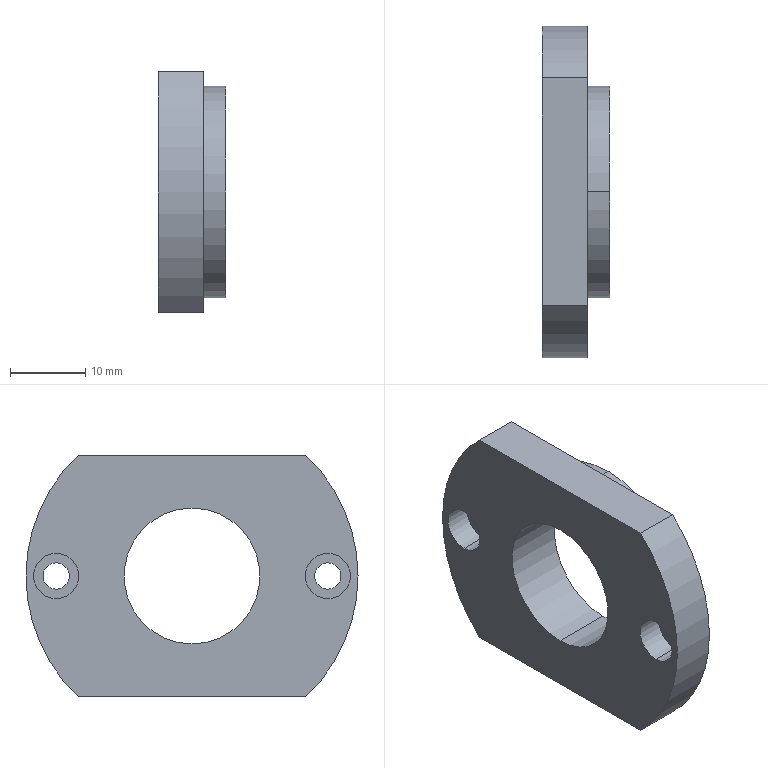Part | SolidWorks | features HoleWzd 1, ICE 1, Revolution 1 | 1 solid | 24 faces | box 9 x 44 x 32 mm | volume 6703 mm3 | cylinder 16 | plane 8 | commonest cylinder face diameters 3.5 x4 6 x4 18 x2 25 x2 28 x2 44 x2
STEP:
#1=CARTESIAN_POINT('',(3.5,18.,-3.));
#2=VERTEX_POINT('',#1);
#3=CARTESIAN_POINT('',(3.5,18.,3.));
#4=VERTEX_POINT('',#3);
#5=CARTESIAN_POINT('',(3.5,18.,0.));
#6=DIRECTION('',(-1.,0.,0.));
#7=DIRECTION('',(0.,0.,1.));
#8=AXIS2_PLACEMENT_3D('',#5,#6,#7);
#9=CIRCLE('',#8,3.);
#10=EDGE_CURVE('',#2,#4,#9,.T.);
#11=ORIENTED_EDGE('',*,*,#10,.F.);
#12=CARTESIAN_POINT('',(0.,18.,-3.));
#13=VERTEX_POINT('',#12);
#14=CARTESIAN_POINT('',(0.,18.,-3.));
#15=DIRECTION('',(-1.,0.,0.));
#16=VECTOR('',#15,1000.);
#17=LINE('',#14,#16);
#18=EDGE_CURVE('',#2,#13,#17,.T.);
#19=ORIENTED_EDGE('',*,*,#18,.T.);
#20=CARTESIAN_POINT('',(0.,18.,3.));
#21=VERTEX_POINT('',#20);
#22=CARTESIAN_POINT('',(0.,18.,0.));
#23=DIRECTION('',(-1.,0.,0.));
#24=DIRECTION('',(0.,0.,1.));
#25=AXIS2_PLACEMENT_3D('',#22,#23,#24);
#26=CIRCLE('',#25,3.);
#27=EDGE_CURVE('',#13,#21,#26,.T.);
#28=ORIENTED_EDGE('',*,*,#27,.T.);
#29=CARTESIAN_POINT('',(0.,18.,3.));
#30=DIRECTION('',(-1.,0.,0.));
#31=VECTOR('',#30,1000.);
#32=LINE('',#29,#31);
#33=EDGE_CURVE('',#4,#21,#32,.T.);
#34=ORIENTED_EDGE('',*,*,#33,.F.);
#35=EDGE_LOOP('',(#11,#19,#28,#34));
#36=FACE_OUTER_BOUND('',#35,.T.);
#37=CARTESIAN_POINT('',(0.,18.,0.));
#38=DIRECTION('',(-1.,0.,0.));
#39=DIRECTION('',(0.,0.,1.));
#40=AXIS2_PLACEMENT_3D('',#37,#38,#39);
#41=CYLINDRICAL_SURFACE('',#40,3.);
#42=ADVANCED_FACE('',(#36),#41,.F.);
#43=CARTESIAN_POINT('',(6.,18.,-1.75));
#44=VERTEX_POINT('',#43);
#45=CARTESIAN_POINT('',(6.,18.,1.75));
#46=VERTEX_POINT('',#45);
#47=CARTESIAN_POINT('',(6.,18.,0.));
#48=DIRECTION('',(-1.,0.,0.));
#49=DIRECTION('',(0.,0.,1.));
#50=AXIS2_PLACEMENT_3D('',#47,#48,#49);
#51=CIRCLE('',#50,1.75);
#52=EDGE_CURVE('',#44,#46,#51,.T.);
#53=ORIENTED_EDGE('',*,*,#52,.F.);
#54=CARTESIAN_POINT('',(3.5,18.,-1.75));
#55=VERTEX_POINT('',#54);
#56=CARTESIAN_POINT('',(0.,18.,-1.75));
#57=DIRECTION('',(-1.,0.,0.));
#58=VECTOR('',#57,1000.);
#59=LINE('',#56,#58);
#60=EDGE_CURVE('',#44,#55,#59,.T.);
#61=ORIENTED_EDGE('',*,*,#60,.T.);
#62=CARTESIAN_POINT('',(3.5,18.,1.75));
#63=VERTEX_POINT('',#62);
#64=CARTESIAN_POINT('',(3.5,18.,0.));
#65=DIRECTION('',(-1.,0.,0.));
#66=DIRECTION('',(0.,0.,1.));
#67=AXIS2_PLACEMENT_3D('',#64,#65,#66);
#68=CIRCLE('',#67,1.75);
#69=EDGE_CURVE('',#55,#63,#68,.T.);
#70=ORIENTED_EDGE('',*,*,#69,.T.);
#71=CARTESIAN_POINT('',(0.,18.,1.75));
#72=DIRECTION('',(-1.,0.,0.));
#73=VECTOR('',#72,1000.);
#74=LINE('',#71,#73);
#75=EDGE_CURVE('',#46,#63,#74,.T.);
#76=ORIENTED_EDGE('',*,*,#75,.F.);
#77=EDGE_LOOP('',(#53,#61,#70,#76));
#78=FACE_OUTER_BOUND('',#77,.T.);
#79=CARTESIAN_POINT('',(0.,18.,0.));
#80=DIRECTION('',(-1.,0.,0.));
#81=DIRECTION('',(0.,0.,1.));
#82=AXIS2_PLACEMENT_3D('',#79,#80,#81);
#83=CYLINDRICAL_SURFACE('',#82,1.75);
#84=ADVANCED_FACE('',(#78),#83,.F.);
#85=CARTESIAN_POINT('',(3.5,-18.,-3.));
#86=VERTEX_POINT('',#85);
#87=CARTESIAN_POINT('',(3.5,-18.,3.));
#88=VERTEX_POINT('',#87);
#89=CARTESIAN_POINT('',(3.5,-18.,0.));
#90=DIRECTION('',(-1.,0.,0.));
#91=DIRECTION('',(0.,0.,1.));
#92=AXIS2_PLACEMENT_3D('',#89,#90,#91);
#93=CIRCLE('',#92,3.);
#94=EDGE_CURVE('',#86,#88,#93,.T.);
#95=ORIENTED_EDGE('',*,*,#94,.F.);
#96=CARTESIAN_POINT('',(0.,-18.,-3.));
#97=VERTEX_POINT('',#96);
#98=CARTESIAN_POINT('',(0.,-18.,-3.));
#99=DIRECTION('',(-1.,0.,0.));
#100=VECTOR('',#99,1000.);
#101=LINE('',#98,#100);
#102=EDGE_CURVE('',#86,#97,#101,.T.);
#103=ORIENTED_EDGE('',*,*,#102,.T.);
#104=CARTESIAN_POINT('',(0.,-18.,3.));
#105=VERTEX_POINT('',#104);
#106=CARTESIAN_POINT('',(0.,-18.,0.));
#107=DIRECTION('',(-1.,0.,0.));
#108=DIRECTION('',(0.,0.,1.));
#109=AXIS2_PLACEMENT_3D('',#106,#107,#108);
#110=CIRCLE('',#109,3.);
#111=EDGE_CURVE('',#97,#105,#110,.T.);
#112=ORIENTED_EDGE('',*,*,#111,.T.);
#113=CARTESIAN_POINT('',(0.,-18.,3.));
#114=DIRECTION('',(-1.,0.,0.));
#115=VECTOR('',#114,1000.);
#116=LINE('',#113,#115);
#117=EDGE_CURVE('',#88,#105,#116,.T.);
#118=ORIENTED_EDGE('',*,*,#117,.F.);
#119=EDGE_LOOP('',(#95,#103,#112,#118));
#120=FACE_OUTER_BOUND('',#119,.T.);
#121=CARTESIAN_POINT('',(0.,-18.,0.));
#122=DIRECTION('',(-1.,0.,0.));
#123=DIRECTION('',(0.,0.,1.));
#124=AXIS2_PLACEMENT_3D('',#121,#122,#123);
#125=CYLINDRICAL_SURFACE('',#124,3.);
#126=ADVANCED_FACE('',(#120),#125,.F.);
#127=CARTESIAN_POINT('',(6.,-18.,-1.75));
#128=VERTEX_POINT('',#127);
#129=CARTESIAN_POINT('',(6.,-18.,1.75));
#130=VERTEX_POINT('',#129);
#131=CARTESIAN_POINT('',(6.,-18.,0.));
#132=DIRECTION('',(-1.,0.,0.));
#133=DIRECTION('',(0.,0.,1.));
#134=AXIS2_PLACEMENT_3D('',#131,#132,#133);
#135=CIRCLE('',#134,1.75);
#136=EDGE_CURVE('',#128,#130,#135,.T.);
#137=ORIENTED_EDGE('',*,*,#136,.F.);
#138=CARTESIAN_POINT('',(3.5,-18.,-1.75));
#139=VERTEX_POINT('',#138);
#140=CARTESIAN_POINT('',(0.,-18.,-1.75));
#141=DIRECTION('',(-1.,0.,0.));
#142=VECTOR('',#141,1000.);
#143=LINE('',#140,#142);
#144=EDGE_CURVE('',#128,#139,#143,.T.);
#145=ORIENTED_EDGE('',*,*,#144,.T.);
#146=CARTESIAN_POINT('',(3.5,-18.,1.75));
#147=VERTEX_POINT('',#146);
#148=CARTESIAN_POINT('',(3.5,-18.,0.));
#149=DIRECTION('',(-1.,0.,0.));
#150=DIRECTION('',(0.,0.,1.));
#151=AXIS2_PLACEMENT_3D('',#148,#149,#150);
#152=CIRCLE('',#151,1.75);
#153=EDGE_CURVE('',#139,#147,#152,.T.);
#154=ORIENTED_EDGE('',*,*,#153,.T.);
#155=CARTESIAN_POINT('',(0.,-18.,1.75));
#156=DIRECTION('',(-1.,0.,0.));
#157=VECTOR('',#156,1000.);
#158=LINE('',#155,#157);
#159=EDGE_CURVE('',#130,#147,#158,.T.);
#160=ORIENTED_EDGE('',*,*,#159,.F.);
#161=EDGE_LOOP('',(#137,#145,#154,#160));
#162=FACE_OUTER_BOUND('',#161,.T.);
#163=CARTESIAN_POINT('',(0.,-18.,0.));
#164=DIRECTION('',(-1.,0.,0.));
#165=DIRECTION('',(0.,0.,1.));
#166=AXIS2_PLACEMENT_3D('',#163,#164,#165);
#167=CYLINDRICAL_SURFACE('',#166,1.75);
#168=ADVANCED_FACE('',(#162),#167,.F.);
#169=CARTESIAN_POINT('',(9.,0.,-12.5));
#170=VERTEX_POINT('',#169);
#171=CARTESIAN_POINT('',(9.,0.,12.5));
#172=VERTEX_POINT('',#171);
#173=CARTESIAN_POINT('',(9.,0.,0.));
#174=DIRECTION('',(-1.,0.,0.));
#175=DIRECTION('',(0.,0.,1.));
#176=AXIS2_PLACEMENT_3D('',#173,#174,#175);
#177=CIRCLE('',#176,12.5);
#178=EDGE_CURVE('',#170,#172,#177,.T.);
#179=ORIENTED_EDGE('',*,*,#178,.F.);
#180=CARTESIAN_POINT('',(8.,0.,-12.5));
#181=VERTEX_POINT('',#180);
#182=CARTESIAN_POINT('',(0.,0.,-12.5));
#183=DIRECTION('',(-1.,0.,0.));
#184=VECTOR('',#183,1000.);
#185=LINE('',#182,#184);
#186=EDGE_CURVE('',#170,#181,#185,.T.);
#187=ORIENTED_EDGE('',*,*,#186,.T.);
#188=CARTESIAN_POINT('',(8.,0.,12.5));
#189=VERTEX_POINT('',#188);
#190=CARTESIAN_POINT('',(8.,0.,0.));
#191=DIRECTION('',(-1.,0.,0.));
#192=DIRECTION('',(0.,0.,1.));
#193=AXIS2_PLACEMENT_3D('',#190,#191,#192);
#194=CIRCLE('',#193,12.5);
#195=EDGE_CURVE('',#181,#189,#194,.T.);
#196=ORIENTED_EDGE('',*,*,#195,.T.);
#197=CARTESIAN_POINT('',(0.,0.,12.5));
#198=DIRECTION('',(-1.,0.,0.));
#199=VECTOR('',#198,1000.);
#200=LINE('',#197,#199);
#201=EDGE_CURVE('',#172,#189,#200,.T.);
#202=ORIENTED_EDGE('',*,*,#201,.F.);
#203=EDGE_LOOP('',(#179,#187,#196,#202));
#204=FACE_OUTER_BOUND('',#203,.T.);
#205=CARTESIAN_POINT('',(0.,0.,0.));
#206=DIRECTION('',(-1.,0.,0.));
#207=DIRECTION('',(0.,0.,1.));
#208=AXIS2_PLACEMENT_3D('',#205,#206,#207);
#209=CYLINDRICAL_SURFACE('',#208,12.5);
#210=ADVANCED_FACE('',(#204),#209,.F.);
#211=CARTESIAN_POINT('',(9.,0.,14.));
#212=VERTEX_POINT('',#211);
#213=CARTESIAN_POINT('',(9.,0.,-14.));
#214=VERTEX_POINT('',#213);
#215=CARTESIAN_POINT('',(9.,0.,0.));
#216=DIRECTION('',(-1.,0.,0.));
#217=DIRECTION('',(0.,0.,1.));
#218=AXIS2_PLACEMENT_3D('',#215,#216,#217);
#219=CIRCLE('',#218,14.);
#220=EDGE_CURVE('',#212,#214,#219,.T.);
#221=ORIENTED_EDGE('',*,*,#220,.T.);
#222=CARTESIAN_POINT('',(6.,0.,-14.));
#223=VERTEX_POINT('',#222);
#224=CARTESIAN_POINT('',(0.,0.,-14.));
#225=DIRECTION('',(-1.,0.,0.));
#226=VECTOR('',#225,1000.);
#227=LINE('',#224,#226);
#228=EDGE_CURVE('',#214,#223,#227,.T.);
#229=ORIENTED_EDGE('',*,*,#228,.T.);
#230=CARTESIAN_POINT('',(6.,0.,14.));
#231=VERTEX_POINT('',#230);
#232=CARTESIAN_POINT('',(6.,0.,0.));
#233=DIRECTION('',(-1.,0.,0.));
#234=DIRECTION('',(0.,0.,1.));
#235=AXIS2_PLACEMENT_3D('',#232,#233,#234);
#236=CIRCLE('',#235,14.);
#237=EDGE_CURVE('',#231,#223,#236,.T.);
#238=ORIENTED_EDGE('',*,*,#237,.F.);
#239=CARTESIAN_POINT('',(0.,0.,14.));
#240=DIRECTION('',(-1.,0.,0.));
#241=VECTOR('',#240,1000.);
#242=LINE('',#239,#241);
#243=EDGE_CURVE('',#212,#231,#242,.T.);
#244=ORIENTED_EDGE('',*,*,#243,.F.);
#245=EDGE_LOOP('',(#221,#229,#238,#244));
#246=FACE_OUTER_BOUND('',#245,.T.);
#247=CARTESIAN_POINT('',(0.,0.,0.));
#248=DIRECTION('',(-1.,0.,0.));
#249=DIRECTION('',(0.,0.,1.));
#250=AXIS2_PLACEMENT_3D('',#247,#248,#249);
#251=CYLINDRICAL_SURFACE('',#250,14.);
#252=ADVANCED_FACE('',(#246),#251,.T.);
#253=CARTESIAN_POINT('',(8.,0.,-9.));
#254=VERTEX_POINT('',#253);
#255=CARTESIAN_POINT('',(8.,0.,9.));
#256=VERTEX_POINT('',#255);
#257=CARTESIAN_POINT('',(8.,0.,0.));
#258=DIRECTION('',(-1.,0.,0.));
#259=DIRECTION('',(0.,0.,1.));
#260=AXIS2_PLACEMENT_3D('',#257,#258,#259);
#261=CIRCLE('',#260,9.);
#262=EDGE_CURVE('',#254,#256,#261,.T.);
#263=ORIENTED_EDGE('',*,*,#262,.F.);
#264=CARTESIAN_POINT('',(0.,0.,-9.));
#265=VERTEX_POINT('',#264);
#266=CARTESIAN_POINT('',(0.,0.,-9.));
#267=DIRECTION('',(-1.,0.,0.));
#268=VECTOR('',#267,1000.);
#269=LINE('',#266,#268);
#270=EDGE_CURVE('',#254,#265,#269,.T.);
#271=ORIENTED_EDGE('',*,*,#270,.T.);
#272=CARTESIAN_POINT('',(0.,0.,9.));
#273=VERTEX_POINT('',#272);
#274=CARTESIAN_POINT('',(0.,0.,0.));
#275=DIRECTION('',(-1.,0.,0.));
#276=DIRECTION('',(0.,0.,1.));
#277=AXIS2_PLACEMENT_3D('',#274,#275,#276);
#278=CIRCLE('',#277,9.);
#279=EDGE_CURVE('',#265,#273,#278,.T.);
#280=ORIENTED_EDGE('',*,*,#279,.T.);
#281=CARTESIAN_POINT('',(0.,0.,9.));
#282=DIRECTION('',(-1.,0.,0.));
#283=VECTOR('',#282,1000.);
#284=LINE('',#281,#283);
#285=EDGE_CURVE('',#256,#273,#284,.T.);
#286=ORIENTED_EDGE('',*,*,#285,.F.);
#287=EDGE_LOOP('',(#263,#271,#280,#286));
#288=FACE_OUTER_BOUND('',#287,.T.);
#289=CARTESIAN_POINT('',(0.,0.,0.));
#290=DIRECTION('',(-1.,0.,0.));
#291=DIRECTION('',(0.,0.,1.));
#292=AXIS2_PLACEMENT_3D('',#289,#290,#291);
#293=CYLINDRICAL_SURFACE('',#292,9.);
#294=ADVANCED_FACE('',(#288),#293,.F.);
#295=CARTESIAN_POINT('',(0.,18.,0.));
#296=DIRECTION('',(-1.,0.,0.));
#297=DIRECTION('',(0.,0.,1.));
#298=AXIS2_PLACEMENT_3D('',#295,#296,#297);
#299=CIRCLE('',#298,3.);
#300=EDGE_CURVE('',#21,#13,#299,.T.);
#301=ORIENTED_EDGE('',*,*,#300,.F.);
#302=ORIENTED_EDGE('',*,*,#27,.F.);
#303=EDGE_LOOP('',(#301,#302));
#304=FACE_BOUND('',#303,.T.);
#305=CARTESIAN_POINT('',(0.,-18.,0.));
#306=DIRECTION('',(-1.,0.,0.));
#307=DIRECTION('',(0.,0.,1.));
#308=AXIS2_PLACEMENT_3D('',#305,#306,#307);
#309=CIRCLE('',#308,3.);
#310=EDGE_CURVE('',#105,#97,#309,.T.);
#311=ORIENTED_EDGE('',*,*,#310,.F.);
#312=ORIENTED_EDGE('',*,*,#111,.F.);
#313=EDGE_LOOP('',(#311,#312));
#314=FACE_BOUND('',#313,.T.);
#315=CARTESIAN_POINT('',(0.,0.,0.));
#316=DIRECTION('',(-1.,0.,0.));
#317=DIRECTION('',(0.,0.,1.));
#318=AXIS2_PLACEMENT_3D('',#315,#316,#317);
#319=CIRCLE('',#318,9.);
#320=EDGE_CURVE('',#273,#265,#319,.T.);
#321=ORIENTED_EDGE('',*,*,#320,.F.);
#322=ORIENTED_EDGE('',*,*,#279,.F.);
#323=EDGE_LOOP('',(#321,#322));
#324=FACE_BOUND('',#323,.T.);
#325=CARTESIAN_POINT('',(0.,-15.1,16.));
#326=VERTEX_POINT('',#325);
#327=CARTESIAN_POINT('',(0.,15.1,16.));
#328=VERTEX_POINT('',#327);
#329=CARTESIAN_POINT('',(0.,25.,16.));
#330=DIRECTION('',(0.,1.,0.));
#331=VECTOR('',#330,1000.);
#332=LINE('',#329,#331);
#333=EDGE_CURVE('',#326,#328,#332,.T.);
#334=ORIENTED_EDGE('',*,*,#333,.T.);
#335=CARTESIAN_POINT('',(0.,15.1,-16.));
#336=VERTEX_POINT('',#335);
#337=CARTESIAN_POINT('',(0.,0.,0.));
#338=DIRECTION('',(-1.,0.,0.));
#339=DIRECTION('',(0.,0.,1.));
#340=AXIS2_PLACEMENT_3D('',#337,#338,#339);
#341=CIRCLE('',#340,22.);
#342=EDGE_CURVE('',#328,#336,#341,.T.);
#343=ORIENTED_EDGE('',*,*,#342,.T.);
#344=CARTESIAN_POINT('',(0.,-15.1,-16.));
#345=VERTEX_POINT('',#344);
#346=CARTESIAN_POINT('',(0.,25.,-16.));
#347=DIRECTION('',(0.,-1.,0.));
#348=VECTOR('',#347,1000.);
#349=LINE('',#346,#348);
#350=EDGE_CURVE('',#336,#345,#349,.T.);
#351=ORIENTED_EDGE('',*,*,#350,.T.);
#352=CARTESIAN_POINT('',(0.,0.,0.));
#353=DIRECTION('',(-1.,0.,0.));
#354=DIRECTION('',(0.,0.,1.));
#355=AXIS2_PLACEMENT_3D('',#352,#353,#354);
#356=CIRCLE('',#355,22.);
#357=EDGE_CURVE('',#345,#326,#356,.T.);
#358=ORIENTED_EDGE('',*,*,#357,.T.);
#359=EDGE_LOOP('',(#334,#343,#351,#358));
#360=FACE_OUTER_BOUND('',#359,.T.);
#361=CARTESIAN_POINT('',(0.,9.,0.));
#362=DIRECTION('',(1.,0.,0.));
#363=DIRECTION('',(0.,0.,-1.));
#364=AXIS2_PLACEMENT_3D('',#361,#362,#363);
#365=PLANE('',#364);
#366=ADVANCED_FACE('',(#304,#314,#324,#360),#365,.F.);
#367=CARTESIAN_POINT('',(6.,15.1,16.));
#368=VERTEX_POINT('',#367);
#369=CARTESIAN_POINT('',(0.,15.1,16.));
#370=DIRECTION('',(-1.,0.,0.));
#371=VECTOR('',#370,1000.);
#372=LINE('',#369,#371);
#373=EDGE_CURVE('',#368,#328,#372,.T.);
#374=ORIENTED_EDGE('',*,*,#373,.F.);
#375=CARTESIAN_POINT('',(6.,15.1,-16.));
#376=VERTEX_POINT('',#375);
#377=CARTESIAN_POINT('',(6.,0.,0.));
#378=DIRECTION('',(-1.,0.,0.));
#379=DIRECTION('',(0.,0.,1.));
#380=AXIS2_PLACEMENT_3D('',#377,#378,#379);
#381=CIRCLE('',#380,22.);
#382=EDGE_CURVE('',#368,#376,#381,.T.);
#383=ORIENTED_EDGE('',*,*,#382,.T.);
#384=CARTESIAN_POINT('',(0.,15.1,-16.));
#385=DIRECTION('',(1.,0.,0.));
#386=VECTOR('',#385,1000.);
#387=LINE('',#384,#386);
#388=EDGE_CURVE('',#336,#376,#387,.T.);
#389=ORIENTED_EDGE('',*,*,#388,.F.);
#390=ORIENTED_EDGE('',*,*,#342,.F.);
#391=EDGE_LOOP('',(#374,#383,#389,#390));
#392=FACE_OUTER_BOUND('',#391,.T.);
#393=CARTESIAN_POINT('',(0.,0.,0.));
#394=DIRECTION('',(-1.,0.,0.));
#395=DIRECTION('',(0.,0.,1.));
#396=AXIS2_PLACEMENT_3D('',#393,#394,#395);
#397=CYLINDRICAL_SURFACE('',#396,22.);
#398=ADVANCED_FACE('',(#392),#397,.T.);
#399=CARTESIAN_POINT('',(6.,-15.1,16.));
#400=VERTEX_POINT('',#399);
#401=CARTESIAN_POINT('',(0.,-15.1,16.));
#402=DIRECTION('',(1.,0.,0.));
#403=VECTOR('',#402,1000.);
#404=LINE('',#401,#403);
#405=EDGE_CURVE('',#326,#400,#404,.T.);
#406=ORIENTED_EDGE('',*,*,#405,.F.);
#407=ORIENTED_EDGE('',*,*,#357,.F.);
#408=CARTESIAN_POINT('',(6.,-15.1,-16.));
#409=VERTEX_POINT('',#408);
#410=CARTESIAN_POINT('',(0.,-15.1,-16.));
#411=DIRECTION('',(-1.,0.,0.));
#412=VECTOR('',#411,1000.);
#413=LINE('',#410,#412);
#414=EDGE_CURVE('',#409,#345,#413,.T.);
#415=ORIENTED_EDGE('',*,*,#414,.F.);
#416=CARTESIAN_POINT('',(6.,0.,0.));
#417=DIRECTION('',(-1.,0.,0.));
#418=DIRECTION('',(0.,0.,1.));
#419=AXIS2_PLACEMENT_3D('',#416,#417,#418);
#420=CIRCLE('',#419,22.);
#421=EDGE_CURVE('',#409,#400,#420,.T.);
#422=ORIENTED_EDGE('',*,*,#421,.T.);
#423=EDGE_LOOP('',(#406,#407,#415,#422));
#424=FACE_OUTER_BOUND('',#423,.T.);
#425=CARTESIAN_POINT('',(0.,0.,0.));
#426=DIRECTION('',(-1.,0.,0.));
#427=DIRECTION('',(0.,0.,1.));
#428=AXIS2_PLACEMENT_3D('',#425,#426,#427);
#429=CYLINDRICAL_SURFACE('',#428,22.);
#430=ADVANCED_FACE('',(#424),#429,.T.);
#431=CARTESIAN_POINT('',(6.,18.,0.));
#432=DIRECTION('',(-1.,0.,0.));
#433=DIRECTION('',(0.,0.,1.));
#434=AXIS2_PLACEMENT_3D('',#431,#432,#433);
#435=CIRCLE('',#434,1.75);
#436=EDGE_CURVE('',#46,#44,#435,.T.);
#437=ORIENTED_EDGE('',*,*,#436,.T.);
#438=ORIENTED_EDGE('',*,*,#52,.T.);
#439=EDGE_LOOP('',(#437,#438));
#440=FACE_BOUND('',#439,.T.);
#441=CARTESIAN_POINT('',(6.,-18.,0.));
#442=DIRECTION('',(-1.,0.,0.));
#443=DIRECTION('',(0.,0.,1.));
#444=AXIS2_PLACEMENT_3D('',#441,#442,#443);
#445=CIRCLE('',#444,1.75);
#446=EDGE_CURVE('',#130,#128,#445,.T.);
#447=ORIENTED_EDGE('',*,*,#446,.T.);
#448=ORIENTED_EDGE('',*,*,#136,.T.);
#449=EDGE_LOOP('',(#447,#448));
#450=FACE_BOUND('',#449,.T.);
#451=ORIENTED_EDGE('',*,*,#237,.T.);
#452=CARTESIAN_POINT('',(6.,0.,0.));
#453=DIRECTION('',(-1.,0.,0.));
#454=DIRECTION('',(0.,0.,1.));
#455=AXIS2_PLACEMENT_3D('',#452,#453,#454);
#456=CIRCLE('',#455,14.);
#457=EDGE_CURVE('',#223,#231,#456,.T.);
#458=ORIENTED_EDGE('',*,*,#457,.T.);
#459=EDGE_LOOP('',(#451,#458));
#460=FACE_BOUND('',#459,.T.);
#461=CARTESIAN_POINT('',(6.,22.,16.));
#462=DIRECTION('',(0.,1.,0.));
#463=VECTOR('',#462,1000.);
#464=LINE('',#461,#463);
#465=EDGE_CURVE('',#400,#368,#464,.T.);
#466=ORIENTED_EDGE('',*,*,#465,.F.);
#467=ORIENTED_EDGE('',*,*,#421,.F.);
#468=CARTESIAN_POINT('',(6.,22.,-16.));
#469=DIRECTION('',(0.,-1.,0.));
#470=VECTOR('',#469,1000.);
#471=LINE('',#468,#470);
#472=EDGE_CURVE('',#376,#409,#471,.T.);
#473=ORIENTED_EDGE('',*,*,#472,.F.);
#474=ORIENTED_EDGE('',*,*,#382,.F.);
#475=EDGE_LOOP('',(#466,#467,#473,#474));
#476=FACE_OUTER_BOUND('',#475,.T.);
#477=CARTESIAN_POINT('',(6.,22.,0.));
#478=DIRECTION('',(-1.,0.,0.));
#479=DIRECTION('',(0.,0.,1.));
#480=AXIS2_PLACEMENT_3D('',#477,#478,#479);
#481=PLANE('',#480);
#482=ADVANCED_FACE('',(#440,#450,#460,#476),#481,.F.);
#483=ORIENTED_EDGE('',*,*,#270,.F.);
#484=CARTESIAN_POINT('',(8.,0.,0.));
#485=DIRECTION('',(-1.,0.,0.));
#486=DIRECTION('',(0.,0.,1.));
#487=AXIS2_PLACEMENT_3D('',#484,#485,#486);
#488=CIRCLE('',#487,9.);
#489=EDGE_CURVE('',#256,#254,#488,.T.);
#490=ORIENTED_EDGE('',*,*,#489,.F.);
#491=ORIENTED_EDGE('',*,*,#285,.T.);
#492=ORIENTED_EDGE('',*,*,#320,.T.);
#493=EDGE_LOOP('',(#483,#490,#491,#492));
#494=FACE_OUTER_BOUND('',#493,.T.);
#495=CARTESIAN_POINT('',(0.,0.,0.));
#496=DIRECTION('',(-1.,0.,0.));
#497=DIRECTION('',(0.,0.,1.));
#498=AXIS2_PLACEMENT_3D('',#495,#496,#497);
#499=CYLINDRICAL_SURFACE('',#498,9.);
#500=ADVANCED_FACE('',(#494),#499,.F.);
#501=ORIENTED_EDGE('',*,*,#228,.F.);
#502=CARTESIAN_POINT('',(9.,0.,0.));
#503=DIRECTION('',(-1.,0.,0.));
#504=DIRECTION('',(0.,0.,1.));
#505=AXIS2_PLACEMENT_3D('',#502,#503,#504);
#506=CIRCLE('',#505,14.);
#507=EDGE_CURVE('',#214,#212,#506,.T.);
#508=ORIENTED_EDGE('',*,*,#507,.T.);
#509=ORIENTED_EDGE('',*,*,#243,.T.);
#510=ORIENTED_EDGE('',*,*,#457,.F.);
#511=EDGE_LOOP('',(#501,#508,#509,#510));
#512=FACE_OUTER_BOUND('',#511,.T.);
#513=CARTESIAN_POINT('',(0.,0.,0.));
#514=DIRECTION('',(-1.,0.,0.));
#515=DIRECTION('',(0.,0.,1.));
#516=AXIS2_PLACEMENT_3D('',#513,#514,#515);
#517=CYLINDRICAL_SURFACE('',#516,14.);
#518=ADVANCED_FACE('',(#512),#517,.T.);
#519=ORIENTED_EDGE('',*,*,#220,.F.);
#520=ORIENTED_EDGE('',*,*,#507,.F.);
#521=EDGE_LOOP('',(#519,#520));
#522=FACE_OUTER_BOUND('',#521,.T.);
#523=CARTESIAN_POINT('',(9.,0.,0.));
#524=DIRECTION('',(-1.,0.,0.));
#525=DIRECTION('',(0.,0.,1.));
#526=AXIS2_PLACEMENT_3D('',#523,#524,#525);
#527=CIRCLE('',#526,12.5);
#528=EDGE_CURVE('',#172,#170,#527,.T.);
#529=ORIENTED_EDGE('',*,*,#528,.T.);
#530=ORIENTED_EDGE('',*,*,#178,.T.);
#531=EDGE_LOOP('',(#529,#530));
#532=FACE_BOUND('',#531,.T.);
#533=CARTESIAN_POINT('',(9.,14.,0.));
#534=DIRECTION('',(-1.,0.,0.));
#535=DIRECTION('',(0.,0.,1.));
#536=AXIS2_PLACEMENT_3D('',#533,#534,#535);
#537=PLANE('',#536);
#538=ADVANCED_FACE('',(#522,#532),#537,.F.);
#539=ORIENTED_EDGE('',*,*,#186,.F.);
#540=ORIENTED_EDGE('',*,*,#528,.F.);
#541=ORIENTED_EDGE('',*,*,#201,.T.);
#542=CARTESIAN_POINT('',(8.,0.,0.));
#543=DIRECTION('',(-1.,0.,0.));
#544=DIRECTION('',(0.,0.,1.));
#545=AXIS2_PLACEMENT_3D('',#542,#543,#544);
#546=CIRCLE('',#545,12.5);
#547=EDGE_CURVE('',#189,#181,#546,.T.);
#548=ORIENTED_EDGE('',*,*,#547,.T.);
#549=EDGE_LOOP('',(#539,#540,#541,#548));
#550=FACE_OUTER_BOUND('',#549,.T.);
#551=CARTESIAN_POINT('',(0.,0.,0.));
#552=DIRECTION('',(-1.,0.,0.));
#553=DIRECTION('',(0.,0.,1.));
#554=AXIS2_PLACEMENT_3D('',#551,#552,#553);
#555=CYLINDRICAL_SURFACE('',#554,12.5);
#556=ADVANCED_FACE('',(#550),#555,.F.);
#557=ORIENTED_EDGE('',*,*,#547,.F.);
#558=ORIENTED_EDGE('',*,*,#195,.F.);
#559=EDGE_LOOP('',(#557,#558));
#560=FACE_OUTER_BOUND('',#559,.T.);
#561=ORIENTED_EDGE('',*,*,#489,.T.);
#562=ORIENTED_EDGE('',*,*,#262,.T.);
#563=EDGE_LOOP('',(#561,#562));
#564=FACE_BOUND('',#563,.T.);
#565=CARTESIAN_POINT('',(8.,12.5,0.));
#566=DIRECTION('',(-1.,0.,0.));
#567=DIRECTION('',(0.,0.,1.));
#568=AXIS2_PLACEMENT_3D('',#565,#566,#567);
#569=PLANE('',#568);
#570=ADVANCED_FACE('',(#560,#564),#569,.F.);
#571=ORIENTED_EDGE('',*,*,#414,.T.);
#572=ORIENTED_EDGE('',*,*,#350,.F.);
#573=ORIENTED_EDGE('',*,*,#388,.T.);
#574=ORIENTED_EDGE('',*,*,#472,.T.);
#575=EDGE_LOOP('',(#571,#572,#573,#574));
#576=FACE_OUTER_BOUND('',#575,.T.);
#577=CARTESIAN_POINT('',(9.,25.,-16.));
#578=DIRECTION('',(0.,0.,-1.));
#579=DIRECTION('',(0.,1.,0.));
#580=AXIS2_PLACEMENT_3D('',#577,#578,#579);
#581=PLANE('',#580);
#582=ADVANCED_FACE('',(#576),#581,.T.);
#583=ORIENTED_EDGE('',*,*,#373,.T.);
#584=ORIENTED_EDGE('',*,*,#333,.F.);
#585=ORIENTED_EDGE('',*,*,#405,.T.);
#586=ORIENTED_EDGE('',*,*,#465,.T.);
#587=EDGE_LOOP('',(#583,#584,#585,#586));
#588=FACE_OUTER_BOUND('',#587,.T.);
#589=CARTESIAN_POINT('',(9.,25.,16.));
#590=DIRECTION('',(0.,0.,1.));
#591=DIRECTION('',(0.,-1.,0.));
#592=AXIS2_PLACEMENT_3D('',#589,#590,#591);
#593=PLANE('',#592);
#594=ADVANCED_FACE('',(#588),#593,.T.);
#595=ORIENTED_EDGE('',*,*,#144,.F.);
#596=ORIENTED_EDGE('',*,*,#446,.F.);
#597=ORIENTED_EDGE('',*,*,#159,.T.);
#598=CARTESIAN_POINT('',(3.5,-18.,0.));
#599=DIRECTION('',(-1.,0.,0.));
#600=DIRECTION('',(0.,0.,1.));
#601=AXIS2_PLACEMENT_3D('',#598,#599,#600);
#602=CIRCLE('',#601,1.75);
#603=EDGE_CURVE('',#147,#139,#602,.T.);
#604=ORIENTED_EDGE('',*,*,#603,.T.);
#605=EDGE_LOOP('',(#595,#596,#597,#604));
#606=FACE_OUTER_BOUND('',#605,.T.);
#607=CARTESIAN_POINT('',(0.,-18.,0.));
#608=DIRECTION('',(-1.,0.,0.));
#609=DIRECTION('',(0.,0.,1.));
#610=AXIS2_PLACEMENT_3D('',#607,#608,#609);
#611=CYLINDRICAL_SURFACE('',#610,1.75);
#612=ADVANCED_FACE('',(#606),#611,.F.);
#613=ORIENTED_EDGE('',*,*,#603,.F.);
#614=ORIENTED_EDGE('',*,*,#153,.F.);
#615=EDGE_LOOP('',(#613,#614));
#616=FACE_BOUND('',#615,.T.);
#617=CARTESIAN_POINT('',(3.5,-18.,0.));
#618=DIRECTION('',(-1.,0.,0.));
#619=DIRECTION('',(0.,0.,1.));
#620=AXIS2_PLACEMENT_3D('',#617,#618,#619);
#621=CIRCLE('',#620,3.);
#622=EDGE_CURVE('',#88,#86,#621,.T.);
#623=ORIENTED_EDGE('',*,*,#622,.T.);
#624=ORIENTED_EDGE('',*,*,#94,.T.);
#625=EDGE_LOOP('',(#623,#624));
#626=FACE_OUTER_BOUND('',#625,.T.);
#627=CARTESIAN_POINT('',(3.5,-16.25,0.));
#628=DIRECTION('',(1.,0.,0.));
#629=DIRECTION('',(0.,0.,-1.));
#630=AXIS2_PLACEMENT_3D('',#627,#628,#629);
#631=PLANE('',#630);
#632=ADVANCED_FACE('',(#616,#626),#631,.F.);
#633=ORIENTED_EDGE('',*,*,#102,.F.);
#634=ORIENTED_EDGE('',*,*,#622,.F.);
#635=ORIENTED_EDGE('',*,*,#117,.T.);
#636=ORIENTED_EDGE('',*,*,#310,.T.);
#637=EDGE_LOOP('',(#633,#634,#635,#636));
#638=FACE_OUTER_BOUND('',#637,.T.);
#639=CARTESIAN_POINT('',(0.,-18.,0.));
#640=DIRECTION('',(-1.,0.,0.));
#641=DIRECTION('',(0.,0.,1.));
#642=AXIS2_PLACEMENT_3D('',#639,#640,#641);
#643=CYLINDRICAL_SURFACE('',#642,3.);
#644=ADVANCED_FACE('',(#638),#643,.F.);
#645=ORIENTED_EDGE('',*,*,#60,.F.);
#646=ORIENTED_EDGE('',*,*,#436,.F.);
#647=ORIENTED_EDGE('',*,*,#75,.T.);
#648=CARTESIAN_POINT('',(3.5,18.,0.));
#649=DIRECTION('',(-1.,0.,0.));
#650=DIRECTION('',(0.,0.,1.));
#651=AXIS2_PLACEMENT_3D('',#648,#649,#650);
#652=CIRCLE('',#651,1.75);
#653=EDGE_CURVE('',#63,#55,#652,.T.);
#654=ORIENTED_EDGE('',*,*,#653,.T.);
#655=EDGE_LOOP('',(#645,#646,#647,#654));
#656=FACE_OUTER_BOUND('',#655,.T.);
#657=CARTESIAN_POINT('',(0.,18.,0.));
#658=DIRECTION('',(-1.,0.,0.));
#659=DIRECTION('',(0.,0.,1.));
#660=AXIS2_PLACEMENT_3D('',#657,#658,#659);
#661=CYLINDRICAL_SURFACE('',#660,1.75);
#662=ADVANCED_FACE('',(#656),#661,.F.);
#663=ORIENTED_EDGE('',*,*,#653,.F.);
#664=ORIENTED_EDGE('',*,*,#69,.F.);
#665=EDGE_LOOP('',(#663,#664));
#666=FACE_BOUND('',#665,.T.);
#667=CARTESIAN_POINT('',(3.5,18.,0.));
#668=DIRECTION('',(-1.,0.,0.));
#669=DIRECTION('',(0.,0.,1.));
#670=AXIS2_PLACEMENT_3D('',#667,#668,#669);
#671=CIRCLE('',#670,3.);
#672=EDGE_CURVE('',#4,#2,#671,.T.);
#673=ORIENTED_EDGE('',*,*,#672,.T.);
#674=ORIENTED_EDGE('',*,*,#10,.T.);
#675=EDGE_LOOP('',(#673,#674));
#676=FACE_OUTER_BOUND('',#675,.T.);
#677=CARTESIAN_POINT('',(3.5,19.75,0.));
#678=DIRECTION('',(1.,0.,0.));
#679=DIRECTION('',(0.,0.,-1.));
#680=AXIS2_PLACEMENT_3D('',#677,#678,#679);
#681=PLANE('',#680);
#682=ADVANCED_FACE('',(#666,#676),#681,.F.);
#683=ORIENTED_EDGE('',*,*,#18,.F.);
#684=ORIENTED_EDGE('',*,*,#672,.F.);
#685=ORIENTED_EDGE('',*,*,#33,.T.);
#686=ORIENTED_EDGE('',*,*,#300,.T.);
#687=EDGE_LOOP('',(#683,#684,#685,#686));
#688=FACE_OUTER_BOUND('',#687,.T.);
#689=CARTESIAN_POINT('',(0.,18.,0.));
#690=DIRECTION('',(-1.,0.,0.));
#691=DIRECTION('',(0.,0.,1.));
#692=AXIS2_PLACEMENT_3D('',#689,#690,#691);
#693=CYLINDRICAL_SURFACE('',#692,3.);
#694=ADVANCED_FACE('',(#688),#693,.F.);
#695=CLOSED_SHELL('',(#42,#84,#126,#168,#210,#252,#294,#366,#398,#430,#482,#500,#518,#538,#556,#570,#582,#594,#612,#632,#644,#662,#682,#694));
#696=MANIFOLD_SOLID_BREP('',#695);
#697=CARTESIAN_POINT('',(0.,0.,0.));
#698=DIRECTION('',(0.,0.,1.));
#699=DIRECTION('',(1.,0.,0.));
#700=AXIS2_PLACEMENT_3D('',#697,#698,#699);
#701=(LENGTH_UNIT()NAMED_UNIT(*)SI_UNIT(.MILLI.,.METRE.));
#702=UNCERTAINTY_MEASURE_WITH_UNIT(LENGTH_MEASURE(0.00001),#701,'','');
#703=(NAMED_UNIT(*)PLANE_ANGLE_UNIT()SI_UNIT($,.RADIAN.));
#704=(NAMED_UNIT(*)SI_UNIT($,.STERADIAN.)SOLID_ANGLE_UNIT());
#705=(GEOMETRIC_REPRESENTATION_CONTEXT(3)GLOBAL_UNCERTAINTY_ASSIGNED_CONTEXT((#702))GLOBAL_UNIT_ASSIGNED_CONTEXT((#701,#703,#704))REPRESENTATION_CONTEXT('',''));
#706=ADVANCED_BREP_SHAPE_REPRESENTATION('',(#696,#700),#705);